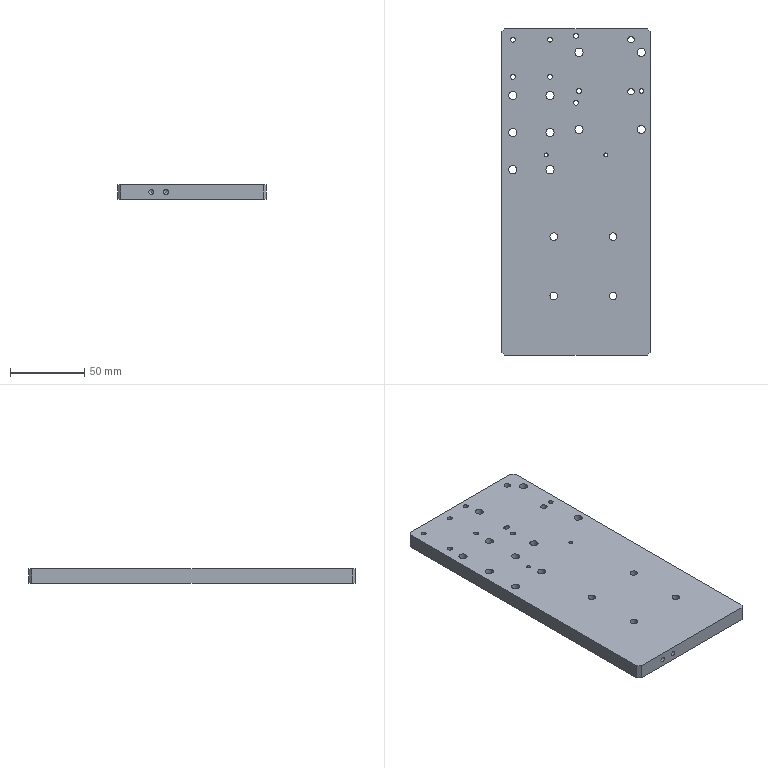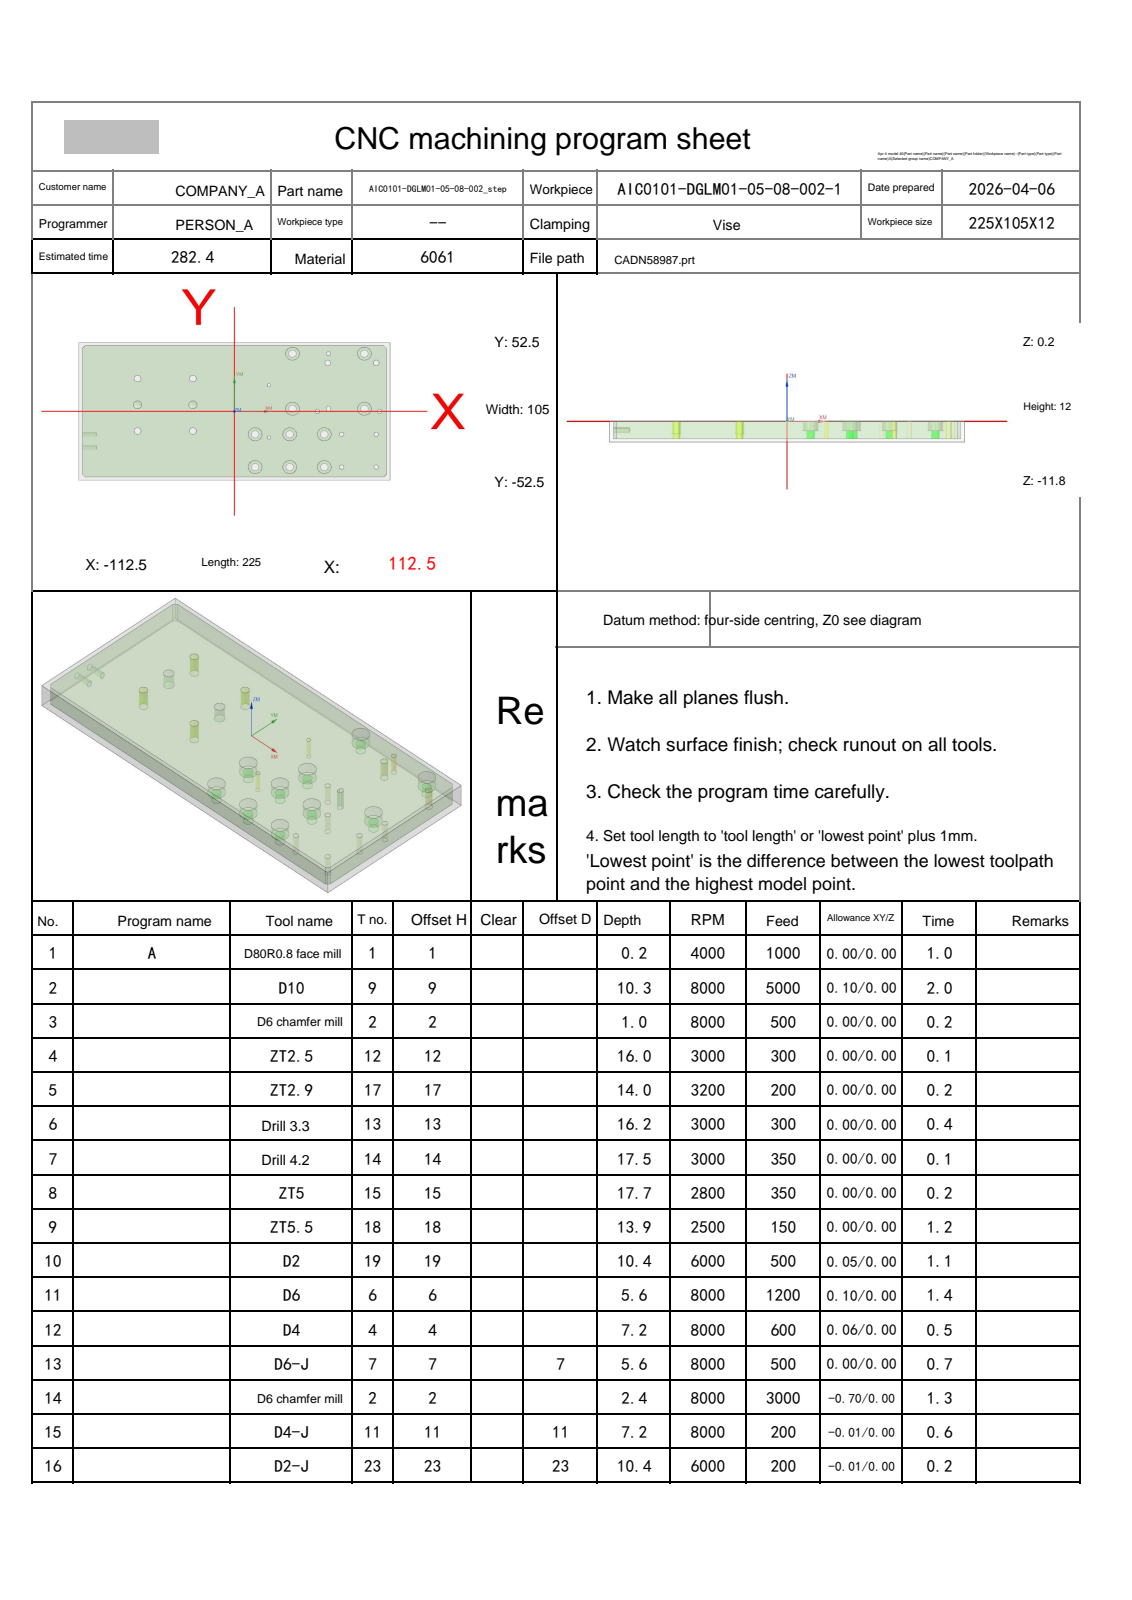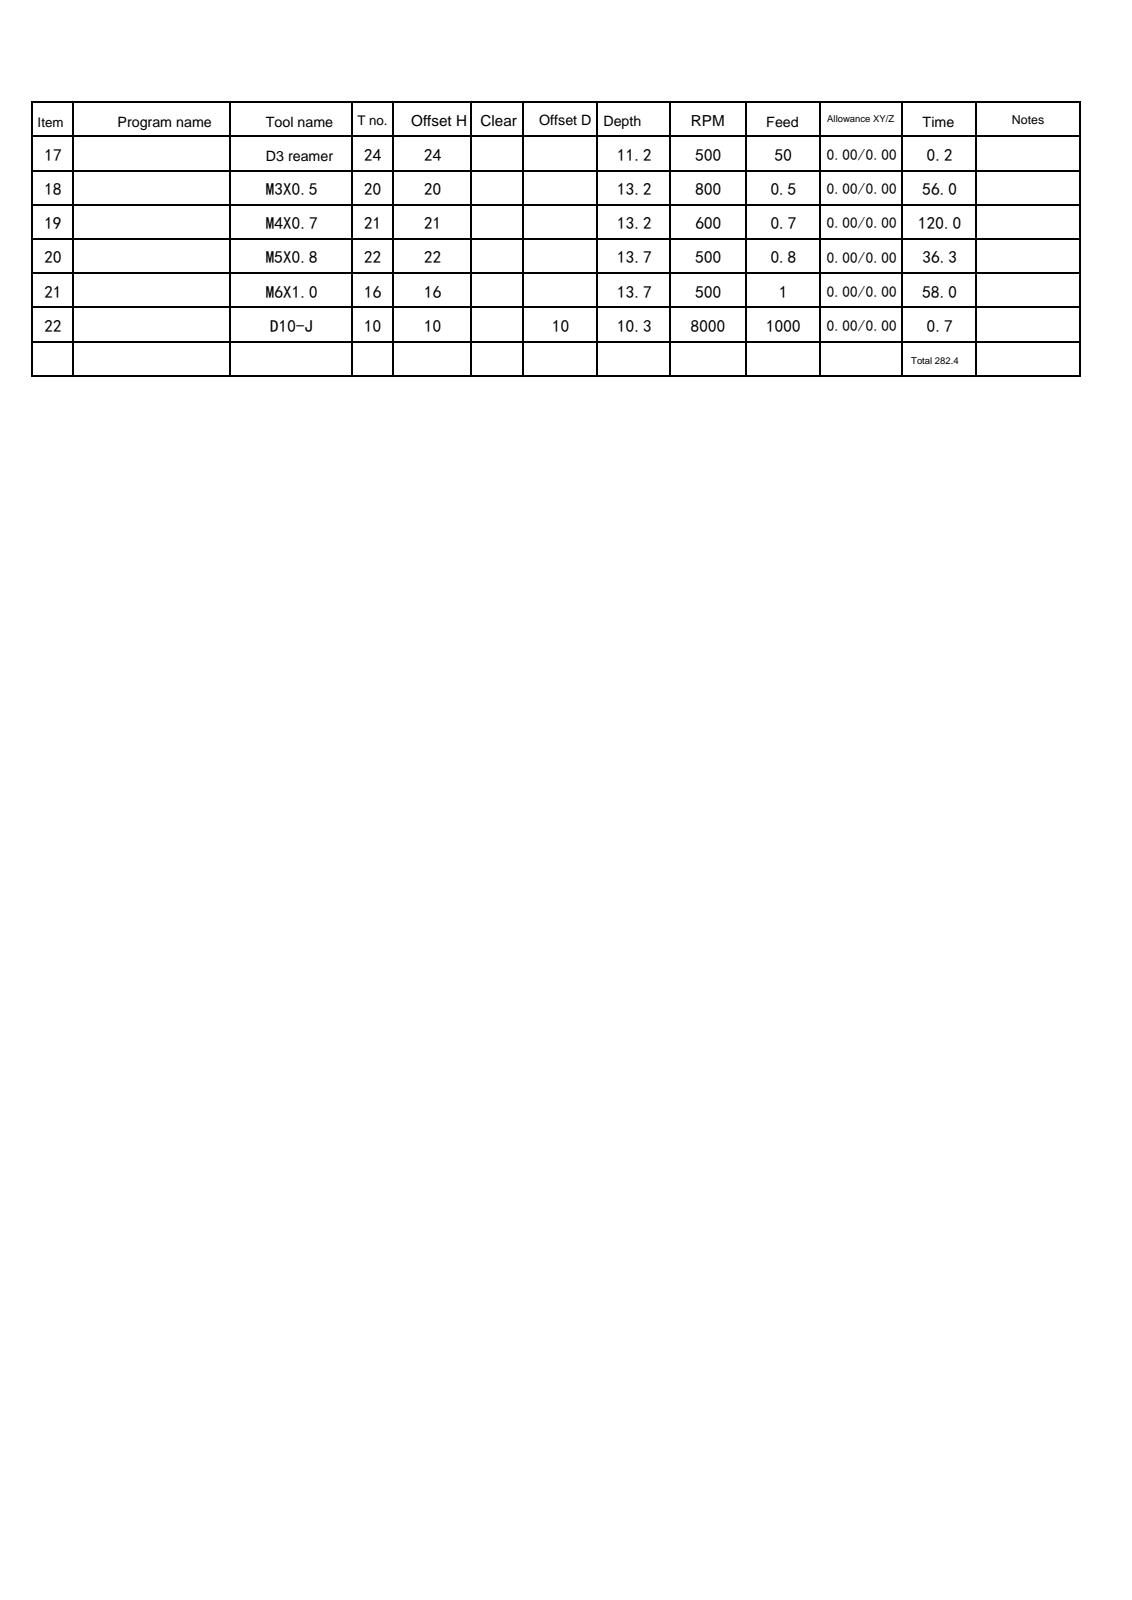NC program | NX | posted by the shop | part box 100 x 220 x 10 mm
Lines 1659 to 2500 of 2500:
N14 T02 M06
(D6 chamfer mill  D=6. R=0. H=02 ce=0.00 di=0.00)
G00 G90 G54 X-.25 Y52.128 M03 S8000
G43 H02 Z20.
M08
Z2.099
G01 Z-1.5 F3000.
G03 X-.33 Y51.828 I.52 J-.3
X-.03 Y51.308 I.6 J0.0
G01 X0.0 Y51.3
X108.
X108.254 Y51.275
X108.497 Y51.201
X108.722 Y51.081
X108.919 Y50.919
X110.919 Y48.919
X111.081 Y48.722
X111.201 Y48.497
X111.275 Y48.254
X111.3 Y48.
Y-48.
X111.275 Y-48.253
X111.201 Y-48.497
X111.081 Y-48.722
X110.919 Y-48.919
X108.919 Y-50.919
X108.722 Y-51.081
X108.497 Y-51.201
X108.254 Y-51.275
X108. Y-51.3
X-108.
X-108.254 Y-51.275
X-108.497 Y-51.201
X-108.722 Y-51.081
X-108.919 Y-50.919
X-110.919 Y-48.919
X-111.081 Y-48.722
X-111.201 Y-48.497
X-111.275 Y-48.254
X-111.3 Y-48.
Y48.
X-111.275 Y48.254
X-111.201 Y48.497
X-111.081 Y48.722
X-110.919 Y48.919
X-108.919 Y50.919
X-108.722 Y51.081
X-108.497 Y51.201
X-108.254 Y51.275
X-108. Y51.3
X0.0
X.03 Y51.308
G03 X.33 Y51.828 I-.3 J.52
X.25 Y52.128 I-.6 J0.0
G01 Z2.099
G00 Z20.
X68.214 Y2.125
Z2.941
G01 Z-1.5
X68.064 Y2.165
G03 X67.804 Y2.015 I0.0 J-.3
G01 X67.8 Y2.
Y1.5
X67.827 Y1.4
X67.9 Y1.327
X68. Y1.3
X68.1 Y1.327
X68.173 Y1.4
X68.2 Y1.5
Y2.5
X68.173 Y2.6
X68.1 Y2.673
X68. Y2.7
X67.9 Y2.673
X67.827 Y2.6
X67.8 Y2.5
Y2.
X67.804 Y1.985
G03 X68.064 Y1.835 I.26 J.15
G01 X68.214 Y1.875
Z2.941
G00 Z20.
G00 G90 X25. Y-20. M03 S8000
Z20.
G98 G81 X25. Y-20. Z-1.75 R3. F500.
Y20.
G80
G00 Z20.
G00 G90 X68. Y44. M03 S8000
Z20.
G98 G81 X68. Y44. Z-1.8 R3. F500.
G80
G00 Z20.
G00 G90 X60. Y0.0 M03 S8000
Z20.
G98 G81 X60. Y0.0 Z-2.2 R3. F500.
X77.5 Y-17.5
Y-42.5
X102.5
Y-17.5
X105. Y0.0
G80
G00 Z20.
G00 G90 X68.194 Y37.093 M03 S8000
Z20.
Z-.5
G01 Z-1. F500.
X69. Y37.2
G03 X67.5 Y38.7 I-1.5 J0.0
X65.8 Y37. I0.0 J-1.7
X67.5 Y35.3 I1.7 J0.0
X69.2 Y37. I0.0 J1.7
X67.5 Y38.7 I-1.7 J0.0
X66. Y37.2 I0.0 J-1.5
G01 X66.806 Y37.093
Z-.5
G00 Z20.
X103.194
Z-.5
G01 Z-1.
X104. Y37.2
G03 X102.5 Y38.7 I-1.5 J0.0
X100.8 Y37. I0.0 J-1.7
X102.5 Y35.3 I1.7 J0.0
X104.2 Y37. I0.0 J1.7
X102.5 Y38.7 I-1.7 J0.0
X101. Y37.2 I0.0 J-1.5
G01 X101.806 Y37.093
Z-.5
G00 Z20.
G00 G90 X-28.979 Y25.409 M03 S8000
Z20.
Z-.6
G01 Z-1.1 F500.
X-28.5 Y25.6
G03 X-30. Y27.1 I-1.5 J0.0
X-32.1 Y25. I0.0 J-2.1
X-30. Y22.9 I2.1 J0.0
X-27.9 Y25. I0.0 J2.1
X-30. Y27.1 I-2.1 J0.0
X-31.5 Y25.6 I0.0 J-1.5
G01 X-31.021 Y25.409
Z-.6
G00 Z20.
X-68.979
Z-.6
G01 Z-1.1
X-68.5 Y25.6
G03 X-70. Y27.1 I-1.5 J0.0
X-72.1 Y25. I0.0 J-2.1
X-70. Y22.9 I2.1 J0.0
X-67.9 Y25. I0.0 J2.1
X-70. Y27.1 I-2.1 J0.0
X-71.5 Y25.6 I0.0 J-1.5
G01 X-71.021 Y25.409
Z-.6
G00 Z20.
X-68.979 Y-14.591
Z-.6
G01 Z-1.1
X-68.5 Y-14.4
G03 X-70. Y-12.9 I-1.5 J0.0
X-72.1 Y-15. I0.0 J-2.1
X-70. Y-17.1 I2.1 J0.0
X-67.9 Y-15. I0.0 J2.1
X-70. Y-12.9 I-2.1 J0.0
X-71.5 Y-14.4 I0.0 J-1.5
G01 X-71.021 Y-14.591
Z-.6
G00 Z20.
X-28.979
Z-.6
G01 Z-1.1
X-28.5 Y-14.4
G03 X-30. Y-12.9 I-1.5 J0.0
X-32.1 Y-15. I0.0 J-2.1
X-30. Y-17.1 I2.1 J0.0
X-27.9 Y-15. I0.0 J2.1
X-30. Y-12.9 I-2.1 J0.0
X-31.5 Y-14.4 I0.0 J-1.5
G01 X-31.021 Y-14.591
Z-.6
G00 Z20.
G00 G90 X-28.853 Y5.612 M03 S8000
Z20.
Z-.5
G01 Z-1. F500.
X-28.5 Y5.8
G03 X-30. Y7.3 I-1.5 J0.0
X-32.3 Y5. I0.0 J-2.3
X-30. Y2.7 I2.3 J0.0
X-27.7 Y5. I0.0 J2.3
X-30. Y7.3 I-2.3 J0.0
X-31.5 Y5.8 I0.0 J-1.5
G01 X-31.147 Y5.612
Z-.5
G00 Z20.
X-68.853
Z-.5
G01 Z-1.
X-68.5 Y5.8
G03 X-70. Y7.3 I-1.5 J0.0
X-72.3 Y5. I0.0 J-2.3
X-70. Y2.7 I2.3 J0.0
X-67.7 Y5. I0.0 J2.3
X-70. Y7.3 I-2.3 J0.0
X-71.5 Y5.8 I0.0 J-1.5
G01 X-71.147 Y5.612
Z-.5
G00 Z20.
G00 G90 X38.614 Y46.654 M03 S8000
Z20.
Z2.5
G01 X38.606 Y46.645 Z2.495 F800.
X38.356 Y46.289 Z2.337
X38.196 Y46.011 Z2.22
X38.012 Y45.617 Z2.062
X37.87 Y45.207 Z1.904
X37.769 Y44.784 Z1.746
X37.712 Y44.354 Z1.588
X37.698 Y43.92 Z1.43
X37.728 Y43.486 Z1.272
X37.801 Y43.058 Z1.114
X37.918 Y42.64 Z.956
X38.076 Y42.235 Z.797
X38.273 Y41.849 Z.639
X38.509 Y41.484 Z.481
X38.781 Y41.145 Z.323
X39.085 Y40.835 Z.165
X39.419 Y40.557 Z.007
X39.779 Y40.314 Z-.151
X40.162 Y40.109 Z-.309
X40.564 Y39.944 Z-.467
X40.98 Y39.82 Z-.625
X41.407 Y39.738 Z-.783
X41.839 Y39.7 Z-.942
X42. Z-1.
G03 X46.3 Y44. I0.0 J4.3
X42. Y48.3 I-4.3 J0.0
X37.7 Y44. I0.0 J-4.3
X42. Y39.7 I4.3 J0.0
X42.499 Y39.729 I0.0 J4.3
G01 Z1.5
G00 Z20.
X38.614 Y4.654
Z2.5
G01 X38.606 Y4.645 Z2.495
X38.356 Y4.289 Z2.337
X38.196 Y4.011 Z2.22
X38.012 Y3.617 Z2.062
X37.87 Y3.207 Z1.904
X37.769 Y2.784 Z1.746
X37.712 Y2.354 Z1.588
X37.698 Y1.92 Z1.43
X37.728 Y1.486 Z1.272
X37.801 Y1.058 Z1.114
X37.918 Y.64 Z.956
X38.076 Y.235 Z.797
X38.273 Y-.152 Z.639
X38.509 Y-.516 Z.481
X38.781 Y-.855 Z.323
X39.085 Y-1.165 Z.165
X39.419 Y-1.443 Z.007
X39.779 Y-1.686 Z-.151
X40.162 Y-1.891 Z-.309
X40.564 Y-2.056 Z-.467
X40.98 Y-2.18 Z-.625
X41.407 Y-2.262 Z-.783
X41.839 Y-2.3 Z-.942
X42. Z-1.
G03 X46.3 Y2. I0.0 J4.3
X42. Y6.3 I-4.3 J0.0
X37.7 Y2. I0.0 J-4.3
X42. Y-2.3 I4.3 J0.0
X42.499 Y-2.271 I0.0 J4.3
G01 Z1.5
G00 Z20.
X36.614 Y-14.846
Z2.5
G01 X36.606 Y-14.855 Z2.495
X36.356 Y-15.211 Z2.337
X36.196 Y-15.489 Z2.22
X36.012 Y-15.883 Z2.062
X35.87 Y-16.293 Z1.904
X35.769 Y-16.716 Z1.746
X35.712 Y-17.146 Z1.588
X35.698 Y-17.58 Z1.43
X35.728 Y-18.014 Z1.272
X35.801 Y-18.442 Z1.114
X35.918 Y-18.86 Z.956
X36.076 Y-19.265 Z.797
X36.273 Y-19.652 Z.639
X36.509 Y-20.016 Z.481
X36.781 Y-20.355 Z.323
X37.085 Y-20.665 Z.165
X37.419 Y-20.943 Z.007
X37.779 Y-21.186 Z-.151
X38.162 Y-21.391 Z-.309
X38.564 Y-21.556 Z-.467
X38.98 Y-21.68 Z-.625
X39.407 Y-21.762 Z-.783
X39.839 Y-21.8 Z-.942
X40. Z-1.
G03 X44.3 Y-17.5 I0.0 J4.3
X40. Y-13.2 I-4.3 J0.0
X35.7 Y-17.5 I0.0 J-4.3
X40. Y-21.8 I4.3 J0.0
X40.499 Y-21.771 I0.0 J4.3
G01 Z1.5
G00 Z20.
X11.614 Y-14.846
Z2.5
G01 X11.606 Y-14.855 Z2.495
X11.356 Y-15.211 Z2.337
X11.196 Y-15.489 Z2.22
X11.012 Y-15.883 Z2.062
X10.87 Y-16.293 Z1.904
X10.769 Y-16.716 Z1.746
X10.712 Y-17.146 Z1.588
X10.698 Y-17.58 Z1.43
X10.728 Y-18.014 Z1.272
X10.801 Y-18.442 Z1.114
X10.918 Y-18.86 Z.956
X11.076 Y-19.265 Z.797
X11.273 Y-19.652 Z.639
X11.509 Y-20.016 Z.481
X11.781 Y-20.355 Z.323
X12.085 Y-20.665 Z.165
X12.419 Y-20.943 Z.007
X12.779 Y-21.186 Z-.151
X13.162 Y-21.391 Z-.309
X13.564 Y-21.556 Z-.467
X13.98 Y-21.68 Z-.625
X14.407 Y-21.762 Z-.783
X14.839 Y-21.8 Z-.942
X15. Z-1.
G03 X19.3 Y-17.5 I0.0 J4.3
X15. Y-13.2 I-4.3 J0.0
X10.7 Y-17.5 I0.0 J-4.3
X15. Y-21.8 I4.3 J0.0
X15.499 Y-21.771 I0.0 J4.3
G01 Z1.5
G00 Z20.
X11.614 Y-39.846
Z2.5
G01 X11.606 Y-39.855 Z2.495
X11.356 Y-40.211 Z2.337
X11.196 Y-40.489 Z2.22
X11.012 Y-40.883 Z2.062
X10.87 Y-41.293 Z1.904
X10.769 Y-41.716 Z1.746
X10.712 Y-42.146 Z1.588
X10.698 Y-42.58 Z1.43
X10.728 Y-43.014 Z1.272
X10.801 Y-43.442 Z1.114
X10.918 Y-43.86 Z.956
X11.076 Y-44.265 Z.797
X11.273 Y-44.652 Z.639
X11.509 Y-45.016 Z.481
X11.781 Y-45.355 Z.323
X12.085 Y-45.665 Z.165
X12.419 Y-45.943 Z.007
X12.779 Y-46.186 Z-.151
X13.162 Y-46.391 Z-.309
X13.564 Y-46.556 Z-.467
X13.98 Y-46.68 Z-.625
X14.407 Y-46.762 Z-.783
X14.839 Y-46.8 Z-.942
X15. Z-1.
G03 X19.3 Y-42.5 I0.0 J4.3
X15. Y-38.2 I-4.3 J0.0
X10.7 Y-42.5 I0.0 J-4.3
X15. Y-46.8 I4.3 J0.0
X15.499 Y-46.771 I0.0 J4.3
G01 Z1.5
G00 Z20.
X36.614 Y-39.846
Z2.5
G01 X36.606 Y-39.855 Z2.495
X36.356 Y-40.211 Z2.337
X36.196 Y-40.489 Z2.22
X36.012 Y-40.883 Z2.062
X35.87 Y-41.293 Z1.904
X35.769 Y-41.716 Z1.746
X35.712 Y-42.146 Z1.588
X35.698 Y-42.58 Z1.43
X35.728 Y-43.014 Z1.272
X35.801 Y-43.442 Z1.114
X35.918 Y-43.86 Z.956
X36.076 Y-44.265 Z.797
X36.273 Y-44.652 Z.639
X36.509 Y-45.016 Z.481
X36.781 Y-45.355 Z.323
X37.085 Y-45.665 Z.165
X37.419 Y-45.943 Z.007
X37.779 Y-46.186 Z-.151
X38.162 Y-46.391 Z-.309
X38.564 Y-46.556 Z-.467
X38.98 Y-46.68 Z-.625
X39.407 Y-46.762 Z-.783
X39.839 Y-46.8 Z-.942
X40. Z-1.
G03 X44.3 Y-42.5 I0.0 J4.3
X40. Y-38.2 I-4.3 J0.0
X35.7 Y-42.5 I0.0 J-4.3
X40. Y-46.8 I4.3 J0.0
X40.499 Y-46.771 I0.0 J4.3
G01 Z1.5
G00 Z20.
X61.614 Y-39.846
Z2.5
G01 X61.606 Y-39.855 Z2.495
X61.356 Y-40.211 Z2.337
X61.196 Y-40.489 Z2.22
X61.012 Y-40.883 Z2.062
X60.87 Y-41.293 Z1.904
X60.769 Y-41.716 Z1.746
X60.712 Y-42.146 Z1.588
X60.698 Y-42.58 Z1.43
X60.728 Y-43.014 Z1.272
X60.801 Y-43.442 Z1.114
X60.918 Y-43.86 Z.956
X61.076 Y-44.265 Z.797
X61.273 Y-44.652 Z.639
X61.509 Y-45.016 Z.481
X61.781 Y-45.355 Z.323
X62.085 Y-45.665 Z.165
X62.419 Y-45.943 Z.007
X62.779 Y-46.186 Z-.151
X63.162 Y-46.391 Z-.309
X63.564 Y-46.556 Z-.467
X63.98 Y-46.68 Z-.625
X64.407 Y-46.762 Z-.783
X64.839 Y-46.8 Z-.942
X65. Z-1.
G03 X69.3 Y-42.5 I0.0 J4.3
X65. Y-38.2 I-4.3 J0.0
X60.7 Y-42.5 I0.0 J-4.3
X65. Y-46.8 I4.3 J0.0
X65.499 Y-46.771 I0.0 J4.3
G01 Z1.5
G00 Z20.
X61.614 Y-14.846
Z2.5
G01 X61.606 Y-14.855 Z2.495
X61.356 Y-15.211 Z2.337
X61.196 Y-15.489 Z2.22
X61.012 Y-15.883 Z2.062
X60.87 Y-16.293 Z1.904
X60.769 Y-16.716 Z1.746
X60.712 Y-17.146 Z1.588
X60.698 Y-17.58 Z1.43
X60.728 Y-18.014 Z1.272
X60.801 Y-18.442 Z1.114
X60.918 Y-18.86 Z.956
X61.076 Y-19.265 Z.797
X61.273 Y-19.652 Z.639
X61.509 Y-20.016 Z.481
X61.781 Y-20.355 Z.323
X62.085 Y-20.665 Z.165
X62.419 Y-20.943 Z.007
X62.779 Y-21.186 Z-.151
X63.162 Y-21.391 Z-.309
X63.564 Y-21.556 Z-.467
X63.98 Y-21.68 Z-.625
X64.407 Y-21.762 Z-.783
X64.839 Y-21.8 Z-.942
X65. Z-1.
G03 X69.3 Y-17.5 I0.0 J4.3
X65. Y-13.2 I-4.3 J0.0
X60.7 Y-17.5 I0.0 J-4.3
X65. Y-21.8 I4.3 J0.0
X65.499 Y-21.771 I0.0 J4.3
G01 Z1.5
G00 Z20.
X90.614 Y4.654
Z2.5
G01 X90.606 Y4.645 Z2.495
X90.356 Y4.289 Z2.337
X90.196 Y4.011 Z2.22
X90.012 Y3.617 Z2.062
X89.87 Y3.207 Z1.904
X89.769 Y2.784 Z1.746
X89.712 Y2.354 Z1.588
X89.698 Y1.92 Z1.43
X89.728 Y1.486 Z1.272
X89.801 Y1.058 Z1.114
X89.918 Y.64 Z.956
X90.076 Y.235 Z.797
X90.273 Y-.152 Z.639
X90.509 Y-.516 Z.481
X90.781 Y-.855 Z.323
X91.085 Y-1.165 Z.165
X91.419 Y-1.443 Z.007
X91.779 Y-1.686 Z-.151
X92.162 Y-1.891 Z-.309
X92.564 Y-2.056 Z-.467
X92.98 Y-2.18 Z-.625
X93.407 Y-2.262 Z-.783
X93.839 Y-2.3 Z-.942
X94. Z-1.
G03 X98.3 Y2. I0.0 J4.3
X94. Y6.3 I-4.3 J0.0
X89.7 Y2. I0.0 J-4.3
X94. Y-2.3 I4.3 J0.0
X94.499 Y-2.271 I0.0 J4.3
G01 Z1.5
G00 Z20.
X90.614 Y46.654
Z2.5
G01 X90.606 Y46.645 Z2.495
X90.356 Y46.289 Z2.337
X90.196 Y46.011 Z2.22
X90.012 Y45.617 Z2.062
X89.87 Y45.207 Z1.904
X89.769 Y44.784 Z1.746
X89.712 Y44.354 Z1.588
X89.698 Y43.92 Z1.43
X89.728 Y43.486 Z1.272
X89.801 Y43.058 Z1.114
X89.918 Y42.64 Z.956
X90.076 Y42.235 Z.797
X90.273 Y41.849 Z.639
X90.509 Y41.484 Z.481
X90.781 Y41.145 Z.323
X91.085 Y40.835 Z.165
X91.419 Y40.557 Z.007
X91.779 Y40.314 Z-.151
X92.162 Y40.109 Z-.309
X92.564 Y39.944 Z-.467
X92.98 Y39.82 Z-.625
X93.407 Y39.738 Z-.783
X93.839 Y39.7 Z-.942
X94. Z-1.
G03 X98.3 Y44. I0.0 J4.3
X94. Y48.3 I-4.3 J0.0
X89.7 Y44. I0.0 J-4.3
X94. Y39.7 I4.3 J0.0
X94.499 Y39.729 I0.0 J4.3
G01 Z1.5
G00 Z20.
G91 G28 Z0.0
M05
M09
G91 G28 Z0.0
M01
N15 T11 M06
(D4-J  D=4. R=0. H=11 ce=-0.01 di=0.00)
G00 G90 G54 X-30. Y5. M03 S8000
G43 H11 Z20.
M08
Z.5
G41 D11
G01 X-29.815 Y5.076 F200.
G03 X-29.515 Y5.525 I-.185 J.449
X-30. Y6.01 I-.485 J0.0
X-30. Y6.01 Z-.5 I0.0 J-1.01
X-30. Y6.01 Z-1.5 I0.0 J-1.01
X-30. Y6.01 Z-2.5 I0.0 J-1.01
X-30. Y6.01 Z-3.5 I0.0 J-1.01
X-30. Y6.01 Z-4.5 I0.0 J-1.01
X-30. Y6.01 Z-5.5 I0.0 J-1.01
X-30. Y6.01 Z-6.5 I0.0 J-1.01
X-30. Y3.99 Z-7. I0.0 J-1.01
X-28.99 Y5. I0.0 J1.01
X-30. Y6.01 I-1.01 J0.0
X-31.01 Y5. I0.0 J-1.01
X-30. Y3.99 I1.01 J0.0
X-29.515 Y4.475 I0.0 J.485
X-29.815 Y4.924 I-.485 J0.0
G01 G40 X-30. Y5.
G00 Z20.
X-70.
Z.5
G41 D11
G01 X-69.815 Y5.076
G03 X-69.515 Y5.525 I-.185 J.449
X-70. Y6.01 I-.485 J0.0
X-70. Y6.01 Z-.5 I0.0 J-1.01
X-70. Y6.01 Z-1.5 I0.0 J-1.01
X-70. Y6.01 Z-2.5 I0.0 J-1.01
X-70. Y6.01 Z-3.5 I0.0 J-1.01
X-70. Y6.01 Z-4.5 I0.0 J-1.01
X-70. Y6.01 Z-5.5 I0.0 J-1.01
X-70. Y6.01 Z-6.5 I0.0 J-1.01
X-70. Y3.99 Z-7. I0.0 J-1.01
X-68.99 Y5. I0.0 J1.01
X-70. Y6.01 I-1.01 J0.0
X-71.01 Y5. I0.0 J-1.01
X-70. Y3.99 I1.01 J0.0
X-69.515 Y4.475 I0.0 J.485
X-69.815 Y4.924 I-.485 J0.0
G01 G40 X-70. Y5.
G00 Z20.
G91 G28 Z0.0
M05
M09
G91 G28 Z0.0
M01
N16 T23 M06
(D2-J  D=2. R=0. H=23 ce=-0.01 di=0.00)
G00 G90 G54 X68.26 Y1.8 M03 S6000
G43 H23 Z20.
M08
Z-1.2
G01 Z-1.7 F200.
G41 D23
X68.31
G03 X68.51 Y2. I0.0 J.2
G01 Y2.5
G03 X68. Y3.01 I-.51 J0.0
X67.49 Y2.5 I0.0 J-.51
G01 Y1.5
G03 X68. Y.99 I.51 J0.0
X68.51 Y1.5 I0.0 J.51
G01 Y2.
Y2.5
G03 X68.31 Y2.7 I-.2 J0.0
G01 X68.237
G40 X68.187
Z-1.2
G00 Z.5
X68.26 Y1.8
Z-2.9
G01 Z-3.4
G41 D23
X68.31
G03 X68.51 Y2. I0.0 J.2
G01 Y2.5
G03 X68. Y3.01 I-.51 J0.0
X67.49 Y2.5 I0.0 J-.51
G01 Y1.5
G03 X68. Y.99 I.51 J0.0
X68.51 Y1.5 I0.0 J.51
G01 Y2.
Y2.5
G03 X68.31 Y2.7 I-.2 J0.0
G01 X68.237
G40 X68.187
Z-2.9
G00 Z-1.2
X68.26 Y1.8
Z-4.6
G01 Z-5.1
G41 D23
X68.31
G03 X68.51 Y2. I0.0 J.2
G01 Y2.5
G03 X68. Y3.01 I-.51 J0.0
X67.49 Y2.5 I0.0 J-.51
G01 Y1.5
G03 X68. Y.99 I.51 J0.0
X68.51 Y1.5 I0.0 J.51
G01 Y2.
Y2.5
G03 X68.31 Y2.7 I-.2 J0.0
G01 X68.237
G40 X68.187
Z-4.6
G00 Z-2.9
X68.26 Y1.8
Z-6.3
G01 Z-6.8
G41 D23
X68.31
G03 X68.51 Y2. I0.0 J.2
G01 Y2.5
G03 X68. Y3.01 I-.51 J0.0
X67.49 Y2.5 I0.0 J-.51
G01 Y1.5
G03 X68. Y.99 I.51 J0.0
X68.51 Y1.5 I0.0 J.51
G01 Y2.
Y2.5
G03 X68.31 Y2.7 I-.2 J0.0
G01 X68.237
G40 X68.187
Z-6.3
G00 Z-4.6
X68.26 Y1.8
Z-8.
G01 Z-8.5
G41 D23
X68.31
G03 X68.51 Y2. I0.0 J.2
G01 Y2.5
G03 X68. Y3.01 I-.51 J0.0
X67.49 Y2.5 I0.0 J-.51
G01 Y1.5
G03 X68. Y.99 I.51 J0.0
X68.51 Y1.5 I0.0 J.51
G01 Y2.
Y2.5
G03 X68.31 Y2.7 I-.2 J0.0
G01 X68.237
G40 X68.187
Z-8.
G00 Z-6.3
X68.26 Y1.8
Z-9.7
G01 Z-10.2
G41 D23
X68.31
G03 X68.51 Y2. I0.0 J.2
G01 Y2.5
G03 X68. Y3.01 I-.51 J0.0
X67.49 Y2.5 I0.0 J-.51
G01 Y1.5
G03 X68. Y.99 I.51 J0.0
X68.51 Y1.5 I0.0 J.51
G01 Y2.
Y2.5
G03 X68.31 Y2.7 I-.2 J0.0
G01 X68.237
G40 X68.187
Z-9.7
G00 Z20.
G91 G28 Z0.0
M05
M09
G91 G28 Z0.0
M01
N17 T24 M06
(D3 reamer D=3. DR_a=180 H=24)
G00 G90 G54 X68. Y44. M03 S500
G43 H24 Z20.
M08
G98 G81 X68. Y44. Z-11. R1. F50.
G80
G00 Z20.
G91 G28 Z0.0
M05
M09
G91 G28 Z0.0
M01
N18 T20 M06
(M3X0.5 D=2.5 DR_a=180 H=20)
G00 G90 G54 X25. Y-20. M03 S800
G43 H20 Z20.
M08
G95
G98 G84 X25. Y-20. Z-13. R1. F.5 Q5.
Y20.
G80
G94
G00 Z20.
G91 G28 Z0.0
M05
M09
G91 G28 Z0.0
M01
N19 T21 M06
(M4X0.7 D=3.3 DR_a=180 H=21)
G00 G90 G54 X60. Y0.0 M03 S600
G43 H21 Z20.
M08
G95
G98 G84 X60. Y0.0 Z-13. R1. F.7 Q4.
X77.5 Y-17.5
Y-42.5
X102.5
Y-17.5
X105. Y0.0
G80
G94
G00 Z20.
G91 G28 Z0.0
M05
M09
G91 G28 Z0.0
M01
N20 T22 M06
(M5X0.8 D=4.2 DR_a=180 H=22)
G00 G90 G54 X67.5 Y37. M03 S500
G43 H22 Z20.
M08
G95
G98 G84 X67.5 Y37. Z-13.5 R1. F.8 Q3.
X102.5
G80
G94
G00 Z20.
G91 G28 Z0.0
M05
M09
G91 G28 Z0.0
M01
N21 T16 M06
(M6X1.0 D=5. DR_a=180 H=16)
G00 G90 G54 X-30. Y25. M03 S500
G43 H16 Z20.
M08
G95
G98 G84 X-30. Y25. Z-13.5 R1. F1. Q3.
X-70.
Y-15.
X-30.
G80
G94
G00 Z20.
G91 G28 Z0.0
M05
M09
G91 G28 Z0.0
M01
N22 T10 M06
(D10-J  D=10. R=0. H=10 ce=0.00 di=0.00)
G00 G90 G54 X-109.013 Y56.116 M03 S8000
G43 H10 Z20.
M08
Z-9.6
G01 Z-10.1 F1000.
G41 D10
X-108.997 Y55.917
G03 X-108. Y55. I.997 J.083
G01 X108.
G02 X111.536 Y53.536 I0.0 J-5.
G01 X113.536 Y51.536
G02 X115. Y48. I-3.536 J-3.536
G01 Y-48.
G02 X113.536 Y-51.536 I-5. J0.0
G01 X111.536 Y-53.536
G02 X108. Y-55. I-3.536 J3.536
G01 X-108.
G02 X-111.536 Y-53.536 I0.0 J5.
G01 X-113.536 Y-51.536
G02 X-115. Y-48. I3.536 J3.536
G01 Y48.
G02 X-113.536 Y51.536 I5. J0.0
G01 X-111.536 Y53.536
G02 X-108. Y55. I3.536 J-3.536
G01 X-107.5
G03 X-106.5 Y56. I0.0 J1.
G01 G40 Y56.2
Z-9.6
G00 Z20.
M05
M09
G91 G28 Z0.0
G91 G28 Y0.0
M30
%